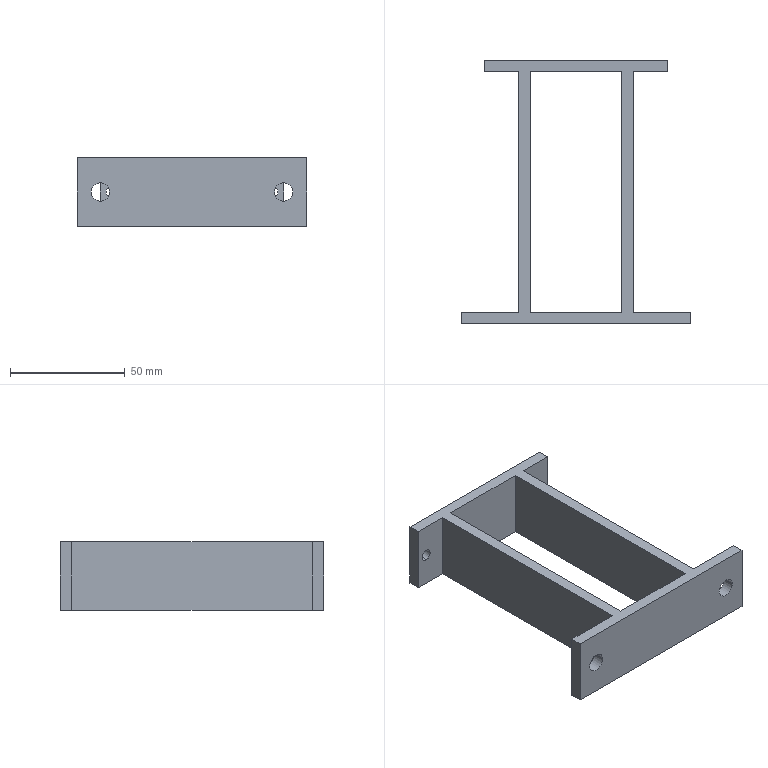Part | SolidWorks | features ICE 2, Extrusion 1 | 1 solid | 26 faces | box 100 x 115 x 30 mm | volume 57801 mm3 | plane 18 | cylinder 8 | commonest cylinder face diameters 5 x4 8 x4
STEP:
#1=CARTESIAN_POINT('',(85.,110.,12.5));
#2=VERTEX_POINT('',#1);
#3=CARTESIAN_POINT('',(85.,110.,17.5));
#4=VERTEX_POINT('',#3);
#5=CARTESIAN_POINT('',(85.,110.,15.));
#6=DIRECTION('',(0.,1.,0.));
#7=DIRECTION('',(0.,0.,1.));
#8=AXIS2_PLACEMENT_3D('',#5,#6,#7);
#9=CIRCLE('',#8,2.5);
#10=EDGE_CURVE('',#2,#4,#9,.T.);
#11=ORIENTED_EDGE('',*,*,#10,.F.);
#12=CARTESIAN_POINT('',(85.,115.,12.5));
#13=VERTEX_POINT('',#12);
#14=CARTESIAN_POINT('',(85.,105.,12.5));
#15=DIRECTION('',(0.,1.,0.));
#16=VECTOR('',#15,1000.);
#17=LINE('',#14,#16);
#18=EDGE_CURVE('',#2,#13,#17,.T.);
#19=ORIENTED_EDGE('',*,*,#18,.T.);
#20=CARTESIAN_POINT('',(85.,115.,17.5));
#21=VERTEX_POINT('',#20);
#22=CARTESIAN_POINT('',(85.,115.,15.));
#23=DIRECTION('',(0.,1.,0.));
#24=DIRECTION('',(0.,0.,1.));
#25=AXIS2_PLACEMENT_3D('',#22,#23,#24);
#26=CIRCLE('',#25,2.5);
#27=EDGE_CURVE('',#13,#21,#26,.T.);
#28=ORIENTED_EDGE('',*,*,#27,.T.);
#29=CARTESIAN_POINT('',(85.,105.,17.5));
#30=DIRECTION('',(0.,1.,0.));
#31=VECTOR('',#30,1000.);
#32=LINE('',#29,#31);
#33=EDGE_CURVE('',#4,#21,#32,.T.);
#34=ORIENTED_EDGE('',*,*,#33,.F.);
#35=EDGE_LOOP('',(#11,#19,#28,#34));
#36=FACE_OUTER_BOUND('',#35,.T.);
#37=CARTESIAN_POINT('',(85.,105.,15.));
#38=DIRECTION('',(0.,1.,0.));
#39=DIRECTION('',(0.,0.,1.));
#40=AXIS2_PLACEMENT_3D('',#37,#38,#39);
#41=CYLINDRICAL_SURFACE('',#40,2.5);
#42=ADVANCED_FACE('',(#36),#41,.F.);
#43=CARTESIAN_POINT('',(15.,110.,12.5));
#44=VERTEX_POINT('',#43);
#45=CARTESIAN_POINT('',(15.,110.,17.5));
#46=VERTEX_POINT('',#45);
#47=CARTESIAN_POINT('',(15.,110.,15.));
#48=DIRECTION('',(0.,1.,0.));
#49=DIRECTION('',(0.,0.,1.));
#50=AXIS2_PLACEMENT_3D('',#47,#48,#49);
#51=CIRCLE('',#50,2.5);
#52=EDGE_CURVE('',#44,#46,#51,.T.);
#53=ORIENTED_EDGE('',*,*,#52,.F.);
#54=CARTESIAN_POINT('',(15.,115.,12.5));
#55=VERTEX_POINT('',#54);
#56=CARTESIAN_POINT('',(15.,105.,12.5));
#57=DIRECTION('',(0.,1.,0.));
#58=VECTOR('',#57,1000.);
#59=LINE('',#56,#58);
#60=EDGE_CURVE('',#44,#55,#59,.T.);
#61=ORIENTED_EDGE('',*,*,#60,.T.);
#62=CARTESIAN_POINT('',(15.,115.,17.5));
#63=VERTEX_POINT('',#62);
#64=CARTESIAN_POINT('',(15.,115.,15.));
#65=DIRECTION('',(0.,1.,0.));
#66=DIRECTION('',(0.,0.,1.));
#67=AXIS2_PLACEMENT_3D('',#64,#65,#66);
#68=CIRCLE('',#67,2.5);
#69=EDGE_CURVE('',#55,#63,#68,.T.);
#70=ORIENTED_EDGE('',*,*,#69,.T.);
#71=CARTESIAN_POINT('',(15.,105.,17.5));
#72=DIRECTION('',(0.,1.,0.));
#73=VECTOR('',#72,1000.);
#74=LINE('',#71,#73);
#75=EDGE_CURVE('',#46,#63,#74,.T.);
#76=ORIENTED_EDGE('',*,*,#75,.F.);
#77=EDGE_LOOP('',(#53,#61,#70,#76));
#78=FACE_OUTER_BOUND('',#77,.T.);
#79=CARTESIAN_POINT('',(15.,105.,15.));
#80=DIRECTION('',(0.,1.,0.));
#81=DIRECTION('',(0.,0.,1.));
#82=AXIS2_PLACEMENT_3D('',#79,#80,#81);
#83=CYLINDRICAL_SURFACE('',#82,2.5);
#84=ADVANCED_FACE('',(#78),#83,.F.);
#85=CARTESIAN_POINT('',(14.,0.,15.));
#86=VERTEX_POINT('',#85);
#87=CARTESIAN_POINT('',(6.,0.,15.));
#88=VERTEX_POINT('',#87);
#89=CARTESIAN_POINT('',(10.,0.,15.));
#90=DIRECTION('',(0.,1.,0.));
#91=DIRECTION('',(-1.,0.,0.));
#92=AXIS2_PLACEMENT_3D('',#89,#90,#91);
#93=CIRCLE('',#92,4.);
#94=EDGE_CURVE('',#86,#88,#93,.T.);
#95=ORIENTED_EDGE('',*,*,#94,.F.);
#96=CARTESIAN_POINT('',(14.,5.,15.));
#97=VERTEX_POINT('',#96);
#98=CARTESIAN_POINT('',(14.,0.,15.));
#99=DIRECTION('',(0.,1.,0.));
#100=VECTOR('',#99,1000.);
#101=LINE('',#98,#100);
#102=EDGE_CURVE('',#86,#97,#101,.T.);
#103=ORIENTED_EDGE('',*,*,#102,.T.);
#104=CARTESIAN_POINT('',(6.,5.,15.));
#105=VERTEX_POINT('',#104);
#106=CARTESIAN_POINT('',(10.,5.,15.));
#107=DIRECTION('',(0.,1.,0.));
#108=DIRECTION('',(-1.,0.,0.));
#109=AXIS2_PLACEMENT_3D('',#106,#107,#108);
#110=CIRCLE('',#109,4.);
#111=EDGE_CURVE('',#97,#105,#110,.T.);
#112=ORIENTED_EDGE('',*,*,#111,.T.);
#113=CARTESIAN_POINT('',(6.,0.,15.));
#114=DIRECTION('',(0.,1.,0.));
#115=VECTOR('',#114,1000.);
#116=LINE('',#113,#115);
#117=EDGE_CURVE('',#88,#105,#116,.T.);
#118=ORIENTED_EDGE('',*,*,#117,.F.);
#119=EDGE_LOOP('',(#95,#103,#112,#118));
#120=FACE_OUTER_BOUND('',#119,.T.);
#121=CARTESIAN_POINT('',(10.,0.,15.));
#122=DIRECTION('',(0.,1.,0.));
#123=DIRECTION('',(-1.,0.,0.));
#124=AXIS2_PLACEMENT_3D('',#121,#122,#123);
#125=CYLINDRICAL_SURFACE('',#124,4.);
#126=ADVANCED_FACE('',(#120),#125,.F.);
#127=CARTESIAN_POINT('',(94.,0.,15.));
#128=VERTEX_POINT('',#127);
#129=CARTESIAN_POINT('',(86.,0.,15.));
#130=VERTEX_POINT('',#129);
#131=CARTESIAN_POINT('',(90.,0.,15.));
#132=DIRECTION('',(0.,1.,0.));
#133=DIRECTION('',(-1.,0.,0.));
#134=AXIS2_PLACEMENT_3D('',#131,#132,#133);
#135=CIRCLE('',#134,4.);
#136=EDGE_CURVE('',#128,#130,#135,.T.);
#137=ORIENTED_EDGE('',*,*,#136,.F.);
#138=CARTESIAN_POINT('',(94.,5.,15.));
#139=VERTEX_POINT('',#138);
#140=CARTESIAN_POINT('',(94.,0.,15.));
#141=DIRECTION('',(0.,1.,0.));
#142=VECTOR('',#141,1000.);
#143=LINE('',#140,#142);
#144=EDGE_CURVE('',#128,#139,#143,.T.);
#145=ORIENTED_EDGE('',*,*,#144,.T.);
#146=CARTESIAN_POINT('',(86.,5.,15.));
#147=VERTEX_POINT('',#146);
#148=CARTESIAN_POINT('',(90.,5.,15.));
#149=DIRECTION('',(0.,1.,0.));
#150=DIRECTION('',(-1.,0.,0.));
#151=AXIS2_PLACEMENT_3D('',#148,#149,#150);
#152=CIRCLE('',#151,4.);
#153=EDGE_CURVE('',#139,#147,#152,.T.);
#154=ORIENTED_EDGE('',*,*,#153,.T.);
#155=CARTESIAN_POINT('',(86.,0.,15.));
#156=DIRECTION('',(0.,1.,0.));
#157=VECTOR('',#156,1000.);
#158=LINE('',#155,#157);
#159=EDGE_CURVE('',#130,#147,#158,.T.);
#160=ORIENTED_EDGE('',*,*,#159,.F.);
#161=EDGE_LOOP('',(#137,#145,#154,#160));
#162=FACE_OUTER_BOUND('',#161,.T.);
#163=CARTESIAN_POINT('',(90.,0.,15.));
#164=DIRECTION('',(0.,1.,0.));
#165=DIRECTION('',(-1.,0.,0.));
#166=AXIS2_PLACEMENT_3D('',#163,#164,#165);
#167=CYLINDRICAL_SURFACE('',#166,4.);
#168=ADVANCED_FACE('',(#162),#167,.F.);
#169=CARTESIAN_POINT('',(0.,5.,30.));
#170=VERTEX_POINT('',#169);
#171=CARTESIAN_POINT('',(0.,0.,30.));
#172=VERTEX_POINT('',#171);
#173=CARTESIAN_POINT('',(0.,5.,30.));
#174=DIRECTION('',(0.,-1.,0.));
#175=VECTOR('',#174,1000.);
#176=LINE('',#173,#175);
#177=EDGE_CURVE('',#170,#172,#176,.T.);
#178=ORIENTED_EDGE('',*,*,#177,.T.);
#179=CARTESIAN_POINT('',(100.,0.,30.));
#180=VERTEX_POINT('',#179);
#181=CARTESIAN_POINT('',(0.,0.,30.));
#182=DIRECTION('',(1.,0.,0.));
#183=VECTOR('',#182,1000.);
#184=LINE('',#181,#183);
#185=EDGE_CURVE('',#172,#180,#184,.T.);
#186=ORIENTED_EDGE('',*,*,#185,.T.);
#187=CARTESIAN_POINT('',(100.,5.,30.));
#188=VERTEX_POINT('',#187);
#189=CARTESIAN_POINT('',(100.,0.,30.));
#190=DIRECTION('',(0.,1.,0.));
#191=VECTOR('',#190,1000.);
#192=LINE('',#189,#191);
#193=EDGE_CURVE('',#180,#188,#192,.T.);
#194=ORIENTED_EDGE('',*,*,#193,.T.);
#195=CARTESIAN_POINT('',(75.,5.,30.));
#196=VERTEX_POINT('',#195);
#197=CARTESIAN_POINT('',(100.,5.,30.));
#198=DIRECTION('',(-1.,0.,0.));
#199=VECTOR('',#198,1000.);
#200=LINE('',#197,#199);
#201=EDGE_CURVE('',#188,#196,#200,.T.);
#202=ORIENTED_EDGE('',*,*,#201,.T.);
#203=CARTESIAN_POINT('',(75.,110.,30.));
#204=VERTEX_POINT('',#203);
#205=CARTESIAN_POINT('',(75.,5.,30.));
#206=DIRECTION('',(0.,1.,0.));
#207=VECTOR('',#206,1000.);
#208=LINE('',#205,#207);
#209=EDGE_CURVE('',#196,#204,#208,.T.);
#210=ORIENTED_EDGE('',*,*,#209,.T.);
#211=CARTESIAN_POINT('',(90.,110.,30.));
#212=VERTEX_POINT('',#211);
#213=CARTESIAN_POINT('',(75.,110.,30.));
#214=DIRECTION('',(1.,0.,0.));
#215=VECTOR('',#214,1000.);
#216=LINE('',#213,#215);
#217=EDGE_CURVE('',#204,#212,#216,.T.);
#218=ORIENTED_EDGE('',*,*,#217,.T.);
#219=CARTESIAN_POINT('',(90.,115.,30.));
#220=VERTEX_POINT('',#219);
#221=CARTESIAN_POINT('',(90.,110.,30.));
#222=DIRECTION('',(0.,1.,0.));
#223=VECTOR('',#222,1000.);
#224=LINE('',#221,#223);
#225=EDGE_CURVE('',#212,#220,#224,.T.);
#226=ORIENTED_EDGE('',*,*,#225,.T.);
#227=CARTESIAN_POINT('',(10.,115.,30.));
#228=VERTEX_POINT('',#227);
#229=CARTESIAN_POINT('',(90.,115.,30.));
#230=DIRECTION('',(-1.,0.,0.));
#231=VECTOR('',#230,1000.);
#232=LINE('',#229,#231);
#233=EDGE_CURVE('',#220,#228,#232,.T.);
#234=ORIENTED_EDGE('',*,*,#233,.T.);
#235=CARTESIAN_POINT('',(10.,110.,30.));
#236=VERTEX_POINT('',#235);
#237=CARTESIAN_POINT('',(10.,115.,30.));
#238=DIRECTION('',(0.,-1.,0.));
#239=VECTOR('',#238,1000.);
#240=LINE('',#237,#239);
#241=EDGE_CURVE('',#228,#236,#240,.T.);
#242=ORIENTED_EDGE('',*,*,#241,.T.);
#243=CARTESIAN_POINT('',(25.,110.,30.));
#244=VERTEX_POINT('',#243);
#245=CARTESIAN_POINT('',(10.,110.,30.));
#246=DIRECTION('',(1.,0.,0.));
#247=VECTOR('',#246,1000.);
#248=LINE('',#245,#247);
#249=EDGE_CURVE('',#236,#244,#248,.T.);
#250=ORIENTED_EDGE('',*,*,#249,.T.);
#251=CARTESIAN_POINT('',(25.,5.,30.));
#252=VERTEX_POINT('',#251);
#253=CARTESIAN_POINT('',(25.,110.,30.));
#254=DIRECTION('',(0.,-1.,0.));
#255=VECTOR('',#254,1000.);
#256=LINE('',#253,#255);
#257=EDGE_CURVE('',#244,#252,#256,.T.);
#258=ORIENTED_EDGE('',*,*,#257,.T.);
#259=CARTESIAN_POINT('',(25.,5.,30.));
#260=DIRECTION('',(-1.,0.,0.));
#261=VECTOR('',#260,1000.);
#262=LINE('',#259,#261);
#263=EDGE_CURVE('',#252,#170,#262,.T.);
#264=ORIENTED_EDGE('',*,*,#263,.T.);
#265=EDGE_LOOP('',(#178,#186,#194,#202,#210,#218,#226,#234,#242,#250,#258,#264));
#266=FACE_OUTER_BOUND('',#265,.T.);
#267=CARTESIAN_POINT('',(30.,5.,30.));
#268=VERTEX_POINT('',#267);
#269=CARTESIAN_POINT('',(70.,5.,30.));
#270=VERTEX_POINT('',#269);
#271=CARTESIAN_POINT('',(30.,5.,30.));
#272=DIRECTION('',(1.,0.,0.));
#273=VECTOR('',#272,1000.);
#274=LINE('',#271,#273);
#275=EDGE_CURVE('',#268,#270,#274,.T.);
#276=ORIENTED_EDGE('',*,*,#275,.F.);
#277=CARTESIAN_POINT('',(30.,110.,30.));
#278=VERTEX_POINT('',#277);
#279=CARTESIAN_POINT('',(30.,110.,30.));
#280=DIRECTION('',(0.,-1.,0.));
#281=VECTOR('',#280,1000.);
#282=LINE('',#279,#281);
#283=EDGE_CURVE('',#278,#268,#282,.T.);
#284=ORIENTED_EDGE('',*,*,#283,.F.);
#285=CARTESIAN_POINT('',(70.,110.,30.));
#286=VERTEX_POINT('',#285);
#287=CARTESIAN_POINT('',(30.,110.,30.));
#288=DIRECTION('',(-1.,0.,0.));
#289=VECTOR('',#288,1000.);
#290=LINE('',#287,#289);
#291=EDGE_CURVE('',#286,#278,#290,.T.);
#292=ORIENTED_EDGE('',*,*,#291,.F.);
#293=CARTESIAN_POINT('',(70.,110.,30.));
#294=DIRECTION('',(0.,1.,0.));
#295=VECTOR('',#294,1000.);
#296=LINE('',#293,#295);
#297=EDGE_CURVE('',#270,#286,#296,.T.);
#298=ORIENTED_EDGE('',*,*,#297,.F.);
#299=EDGE_LOOP('',(#276,#284,#292,#298));
#300=FACE_BOUND('',#299,.T.);
#301=CARTESIAN_POINT('',(0.,0.,30.));
#302=DIRECTION('',(0.,0.,1.));
#303=DIRECTION('',(1.,0.,0.));
#304=AXIS2_PLACEMENT_3D('',#301,#302,#303);
#305=PLANE('',#304);
#306=ADVANCED_FACE('',(#266,#300),#305,.T.);
#307=CARTESIAN_POINT('',(0.,5.,0.));
#308=VERTEX_POINT('',#307);
#309=CARTESIAN_POINT('',(0.,0.,0.));
#310=VERTEX_POINT('',#309);
#311=CARTESIAN_POINT('',(0.,5.,0.));
#312=DIRECTION('',(0.,-1.,0.));
#313=VECTOR('',#312,1000.);
#314=LINE('',#311,#313);
#315=EDGE_CURVE('',#308,#310,#314,.T.);
#316=ORIENTED_EDGE('',*,*,#315,.F.);
#317=CARTESIAN_POINT('',(25.,5.,0.));
#318=VERTEX_POINT('',#317);
#319=CARTESIAN_POINT('',(25.,5.,0.));
#320=DIRECTION('',(-1.,0.,0.));
#321=VECTOR('',#320,1000.);
#322=LINE('',#319,#321);
#323=EDGE_CURVE('',#318,#308,#322,.T.);
#324=ORIENTED_EDGE('',*,*,#323,.F.);
#325=CARTESIAN_POINT('',(25.,110.,0.));
#326=VERTEX_POINT('',#325);
#327=CARTESIAN_POINT('',(25.,110.,0.));
#328=DIRECTION('',(0.,-1.,0.));
#329=VECTOR('',#328,1000.);
#330=LINE('',#327,#329);
#331=EDGE_CURVE('',#326,#318,#330,.T.);
#332=ORIENTED_EDGE('',*,*,#331,.F.);
#333=CARTESIAN_POINT('',(10.,110.,0.));
#334=VERTEX_POINT('',#333);
#335=CARTESIAN_POINT('',(10.,110.,0.));
#336=DIRECTION('',(1.,0.,0.));
#337=VECTOR('',#336,1000.);
#338=LINE('',#335,#337);
#339=EDGE_CURVE('',#334,#326,#338,.T.);
#340=ORIENTED_EDGE('',*,*,#339,.F.);
#341=CARTESIAN_POINT('',(10.,115.,0.));
#342=VERTEX_POINT('',#341);
#343=CARTESIAN_POINT('',(10.,115.,0.));
#344=DIRECTION('',(0.,-1.,0.));
#345=VECTOR('',#344,1000.);
#346=LINE('',#343,#345);
#347=EDGE_CURVE('',#342,#334,#346,.T.);
#348=ORIENTED_EDGE('',*,*,#347,.F.);
#349=CARTESIAN_POINT('',(90.,115.,0.));
#350=VERTEX_POINT('',#349);
#351=CARTESIAN_POINT('',(90.,115.,0.));
#352=DIRECTION('',(-1.,0.,0.));
#353=VECTOR('',#352,1000.);
#354=LINE('',#351,#353);
#355=EDGE_CURVE('',#350,#342,#354,.T.);
#356=ORIENTED_EDGE('',*,*,#355,.F.);
#357=CARTESIAN_POINT('',(90.,110.,0.));
#358=VERTEX_POINT('',#357);
#359=CARTESIAN_POINT('',(90.,110.,0.));
#360=DIRECTION('',(0.,1.,0.));
#361=VECTOR('',#360,1000.);
#362=LINE('',#359,#361);
#363=EDGE_CURVE('',#358,#350,#362,.T.);
#364=ORIENTED_EDGE('',*,*,#363,.F.);
#365=CARTESIAN_POINT('',(75.,110.,0.));
#366=VERTEX_POINT('',#365);
#367=CARTESIAN_POINT('',(75.,110.,0.));
#368=DIRECTION('',(1.,0.,0.));
#369=VECTOR('',#368,1000.);
#370=LINE('',#367,#369);
#371=EDGE_CURVE('',#366,#358,#370,.T.);
#372=ORIENTED_EDGE('',*,*,#371,.F.);
#373=CARTESIAN_POINT('',(75.,5.,0.));
#374=VERTEX_POINT('',#373);
#375=CARTESIAN_POINT('',(75.,5.,0.));
#376=DIRECTION('',(0.,1.,0.));
#377=VECTOR('',#376,1000.);
#378=LINE('',#375,#377);
#379=EDGE_CURVE('',#374,#366,#378,.T.);
#380=ORIENTED_EDGE('',*,*,#379,.F.);
#381=CARTESIAN_POINT('',(100.,5.,0.));
#382=VERTEX_POINT('',#381);
#383=CARTESIAN_POINT('',(100.,5.,0.));
#384=DIRECTION('',(-1.,0.,0.));
#385=VECTOR('',#384,1000.);
#386=LINE('',#383,#385);
#387=EDGE_CURVE('',#382,#374,#386,.T.);
#388=ORIENTED_EDGE('',*,*,#387,.F.);
#389=CARTESIAN_POINT('',(100.,0.,0.));
#390=VERTEX_POINT('',#389);
#391=CARTESIAN_POINT('',(100.,0.,0.));
#392=DIRECTION('',(0.,1.,0.));
#393=VECTOR('',#392,1000.);
#394=LINE('',#391,#393);
#395=EDGE_CURVE('',#390,#382,#394,.T.);
#396=ORIENTED_EDGE('',*,*,#395,.F.);
#397=CARTESIAN_POINT('',(0.,0.,0.));
#398=DIRECTION('',(1.,0.,0.));
#399=VECTOR('',#398,1000.);
#400=LINE('',#397,#399);
#401=EDGE_CURVE('',#310,#390,#400,.T.);
#402=ORIENTED_EDGE('',*,*,#401,.F.);
#403=EDGE_LOOP('',(#316,#324,#332,#340,#348,#356,#364,#372,#380,#388,#396,#402));
#404=FACE_OUTER_BOUND('',#403,.T.);
#405=CARTESIAN_POINT('',(30.,110.,0.));
#406=VERTEX_POINT('',#405);
#407=CARTESIAN_POINT('',(30.,5.,0.));
#408=VERTEX_POINT('',#407);
#409=CARTESIAN_POINT('',(30.,110.,0.));
#410=DIRECTION('',(0.,-1.,0.));
#411=VECTOR('',#410,1000.);
#412=LINE('',#409,#411);
#413=EDGE_CURVE('',#406,#408,#412,.T.);
#414=ORIENTED_EDGE('',*,*,#413,.T.);
#415=CARTESIAN_POINT('',(70.,5.,0.));
#416=VERTEX_POINT('',#415);
#417=CARTESIAN_POINT('',(30.,5.,0.));
#418=DIRECTION('',(1.,0.,0.));
#419=VECTOR('',#418,1000.);
#420=LINE('',#417,#419);
#421=EDGE_CURVE('',#408,#416,#420,.T.);
#422=ORIENTED_EDGE('',*,*,#421,.T.);
#423=CARTESIAN_POINT('',(70.,110.,0.));
#424=VERTEX_POINT('',#423);
#425=CARTESIAN_POINT('',(70.,110.,0.));
#426=DIRECTION('',(0.,1.,0.));
#427=VECTOR('',#426,1000.);
#428=LINE('',#425,#427);
#429=EDGE_CURVE('',#416,#424,#428,.T.);
#430=ORIENTED_EDGE('',*,*,#429,.T.);
#431=CARTESIAN_POINT('',(30.,110.,0.));
#432=DIRECTION('',(-1.,0.,0.));
#433=VECTOR('',#432,1000.);
#434=LINE('',#431,#433);
#435=EDGE_CURVE('',#424,#406,#434,.T.);
#436=ORIENTED_EDGE('',*,*,#435,.T.);
#437=EDGE_LOOP('',(#414,#422,#430,#436));
#438=FACE_BOUND('',#437,.T.);
#439=CARTESIAN_POINT('',(0.,0.,0.));
#440=DIRECTION('',(0.,0.,1.));
#441=DIRECTION('',(1.,0.,0.));
#442=AXIS2_PLACEMENT_3D('',#439,#440,#441);
#443=PLANE('',#442);
#444=ADVANCED_FACE('',(#404,#438),#443,.F.);
#445=ORIENTED_EDGE('',*,*,#315,.T.);
#446=CARTESIAN_POINT('',(0.,0.,30.));
#447=DIRECTION('',(0.,0.,-1.));
#448=VECTOR('',#447,1000.);
#449=LINE('',#446,#448);
#450=EDGE_CURVE('',#172,#310,#449,.T.);
#451=ORIENTED_EDGE('',*,*,#450,.F.);
#452=ORIENTED_EDGE('',*,*,#177,.F.);
#453=CARTESIAN_POINT('',(0.,5.,30.));
#454=DIRECTION('',(0.,0.,-1.));
#455=VECTOR('',#454,1000.);
#456=LINE('',#453,#455);
#457=EDGE_CURVE('',#170,#308,#456,.T.);
#458=ORIENTED_EDGE('',*,*,#457,.T.);
#459=EDGE_LOOP('',(#445,#451,#452,#458));
#460=FACE_OUTER_BOUND('',#459,.T.);
#461=CARTESIAN_POINT('',(0.,5.,30.));
#462=DIRECTION('',(1.,0.,0.));
#463=DIRECTION('',(0.,1.,0.));
#464=AXIS2_PLACEMENT_3D('',#461,#462,#463);
#465=PLANE('',#464);
#466=ADVANCED_FACE('',(#460),#465,.F.);
#467=CARTESIAN_POINT('',(10.,0.,15.));
#468=DIRECTION('',(0.,1.,0.));
#469=DIRECTION('',(-1.,0.,0.));
#470=AXIS2_PLACEMENT_3D('',#467,#468,#469);
#471=CIRCLE('',#470,4.);
#472=EDGE_CURVE('',#88,#86,#471,.T.);
#473=ORIENTED_EDGE('',*,*,#472,.T.);
#474=ORIENTED_EDGE('',*,*,#94,.T.);
#475=EDGE_LOOP('',(#473,#474));
#476=FACE_BOUND('',#475,.T.);
#477=CARTESIAN_POINT('',(90.,0.,15.));
#478=DIRECTION('',(0.,1.,0.));
#479=DIRECTION('',(-1.,0.,0.));
#480=AXIS2_PLACEMENT_3D('',#477,#478,#479);
#481=CIRCLE('',#480,4.);
#482=EDGE_CURVE('',#130,#128,#481,.T.);
#483=ORIENTED_EDGE('',*,*,#482,.T.);
#484=ORIENTED_EDGE('',*,*,#136,.T.);
#485=EDGE_LOOP('',(#483,#484));
#486=FACE_BOUND('',#485,.T.);
#487=ORIENTED_EDGE('',*,*,#401,.T.);
#488=CARTESIAN_POINT('',(100.,0.,30.));
#489=DIRECTION('',(0.,0.,-1.));
#490=VECTOR('',#489,1000.);
#491=LINE('',#488,#490);
#492=EDGE_CURVE('',#180,#390,#491,.T.);
#493=ORIENTED_EDGE('',*,*,#492,.F.);
#494=ORIENTED_EDGE('',*,*,#185,.F.);
#495=ORIENTED_EDGE('',*,*,#450,.T.);
#496=EDGE_LOOP('',(#487,#493,#494,#495));
#497=FACE_OUTER_BOUND('',#496,.T.);
#498=CARTESIAN_POINT('',(0.,0.,30.));
#499=DIRECTION('',(0.,1.,0.));
#500=DIRECTION('',(0.,0.,1.));
#501=AXIS2_PLACEMENT_3D('',#498,#499,#500);
#502=PLANE('',#501);
#503=ADVANCED_FACE('',(#476,#486,#497),#502,.F.);
#504=ORIENTED_EDGE('',*,*,#395,.T.);
#505=CARTESIAN_POINT('',(100.,5.,30.));
#506=DIRECTION('',(0.,0.,-1.));
#507=VECTOR('',#506,1000.);
#508=LINE('',#505,#507);
#509=EDGE_CURVE('',#188,#382,#508,.T.);
#510=ORIENTED_EDGE('',*,*,#509,.F.);
#511=ORIENTED_EDGE('',*,*,#193,.F.);
#512=ORIENTED_EDGE('',*,*,#492,.T.);
#513=EDGE_LOOP('',(#504,#510,#511,#512));
#514=FACE_OUTER_BOUND('',#513,.T.);
#515=CARTESIAN_POINT('',(100.,0.,30.));
#516=DIRECTION('',(-1.,0.,0.));
#517=DIRECTION('',(0.,0.,1.));
#518=AXIS2_PLACEMENT_3D('',#515,#516,#517);
#519=PLANE('',#518);
#520=ADVANCED_FACE('',(#514),#519,.F.);
#521=CARTESIAN_POINT('',(90.,5.,15.));
#522=DIRECTION('',(0.,1.,0.));
#523=DIRECTION('',(-1.,0.,0.));
#524=AXIS2_PLACEMENT_3D('',#521,#522,#523);
#525=CIRCLE('',#524,4.);
#526=EDGE_CURVE('',#147,#139,#525,.T.);
#527=ORIENTED_EDGE('',*,*,#526,.F.);
#528=ORIENTED_EDGE('',*,*,#153,.F.);
#529=EDGE_LOOP('',(#527,#528));
#530=FACE_BOUND('',#529,.T.);
#531=ORIENTED_EDGE('',*,*,#387,.T.);
#532=CARTESIAN_POINT('',(75.,5.,30.));
#533=DIRECTION('',(0.,0.,-1.));
#534=VECTOR('',#533,1000.);
#535=LINE('',#532,#534);
#536=EDGE_CURVE('',#196,#374,#535,.T.);
#537=ORIENTED_EDGE('',*,*,#536,.F.);
#538=ORIENTED_EDGE('',*,*,#201,.F.);
#539=ORIENTED_EDGE('',*,*,#509,.T.);
#540=EDGE_LOOP('',(#531,#537,#538,#539));
#541=FACE_OUTER_BOUND('',#540,.T.);
#542=CARTESIAN_POINT('',(100.,5.,30.));
#543=DIRECTION('',(0.,-1.,0.));
#544=DIRECTION('',(1.,0.,0.));
#545=AXIS2_PLACEMENT_3D('',#542,#543,#544);
#546=PLANE('',#545);
#547=ADVANCED_FACE('',(#530,#541),#546,.F.);
#548=ORIENTED_EDGE('',*,*,#379,.T.);
#549=CARTESIAN_POINT('',(75.,110.,30.));
#550=DIRECTION('',(0.,0.,-1.));
#551=VECTOR('',#550,1000.);
#552=LINE('',#549,#551);
#553=EDGE_CURVE('',#204,#366,#552,.T.);
#554=ORIENTED_EDGE('',*,*,#553,.F.);
#555=ORIENTED_EDGE('',*,*,#209,.F.);
#556=ORIENTED_EDGE('',*,*,#536,.T.);
#557=EDGE_LOOP('',(#548,#554,#555,#556));
#558=FACE_OUTER_BOUND('',#557,.T.);
#559=CARTESIAN_POINT('',(75.,5.,30.));
#560=DIRECTION('',(-1.,0.,0.));
#561=DIRECTION('',(0.,0.,1.));
#562=AXIS2_PLACEMENT_3D('',#559,#560,#561);
#563=PLANE('',#562);
#564=ADVANCED_FACE('',(#558),#563,.F.);
#565=CARTESIAN_POINT('',(85.,110.,15.));
#566=DIRECTION('',(0.,1.,0.));
#567=DIRECTION('',(0.,0.,1.));
#568=AXIS2_PLACEMENT_3D('',#565,#566,#567);
#569=CIRCLE('',#568,2.5);
#570=EDGE_CURVE('',#4,#2,#569,.T.);
#571=ORIENTED_EDGE('',*,*,#570,.T.);
#572=ORIENTED_EDGE('',*,*,#10,.T.);
#573=EDGE_LOOP('',(#571,#572));
#574=FACE_BOUND('',#573,.T.);
#575=ORIENTED_EDGE('',*,*,#371,.T.);
#576=CARTESIAN_POINT('',(90.,110.,30.));
#577=DIRECTION('',(0.,0.,-1.));
#578=VECTOR('',#577,1000.);
#579=LINE('',#576,#578);
#580=EDGE_CURVE('',#212,#358,#579,.T.);
#581=ORIENTED_EDGE('',*,*,#580,.F.);
#582=ORIENTED_EDGE('',*,*,#217,.F.);
#583=ORIENTED_EDGE('',*,*,#553,.T.);
#584=EDGE_LOOP('',(#575,#581,#582,#583));
#585=FACE_OUTER_BOUND('',#584,.T.);
#586=CARTESIAN_POINT('',(75.,110.,30.));
#587=DIRECTION('',(0.,1.,0.));
#588=DIRECTION('',(0.,0.,1.));
#589=AXIS2_PLACEMENT_3D('',#586,#587,#588);
#590=PLANE('',#589);
#591=ADVANCED_FACE('',(#574,#585),#590,.F.);
#592=ORIENTED_EDGE('',*,*,#363,.T.);
#593=CARTESIAN_POINT('',(90.,115.,30.));
#594=DIRECTION('',(0.,0.,-1.));
#595=VECTOR('',#594,1000.);
#596=LINE('',#593,#595);
#597=EDGE_CURVE('',#220,#350,#596,.T.);
#598=ORIENTED_EDGE('',*,*,#597,.F.);
#599=ORIENTED_EDGE('',*,*,#225,.F.);
#600=ORIENTED_EDGE('',*,*,#580,.T.);
#601=EDGE_LOOP('',(#592,#598,#599,#600));
#602=FACE_OUTER_BOUND('',#601,.T.);
#603=CARTESIAN_POINT('',(90.,110.,30.));
#604=DIRECTION('',(-1.,0.,0.));
#605=DIRECTION('',(0.,0.,1.));
#606=AXIS2_PLACEMENT_3D('',#603,#604,#605);
#607=PLANE('',#606);
#608=ADVANCED_FACE('',(#602),#607,.F.);
#609=CARTESIAN_POINT('',(85.,115.,15.));
#610=DIRECTION('',(0.,1.,0.));
#611=DIRECTION('',(0.,0.,1.));
#612=AXIS2_PLACEMENT_3D('',#609,#610,#611);
#613=CIRCLE('',#612,2.5);
#614=EDGE_CURVE('',#21,#13,#613,.T.);
#615=ORIENTED_EDGE('',*,*,#614,.F.);
#616=ORIENTED_EDGE('',*,*,#27,.F.);
#617=EDGE_LOOP('',(#615,#616));
#618=FACE_BOUND('',#617,.T.);
#619=CARTESIAN_POINT('',(15.,115.,15.));
#620=DIRECTION('',(0.,1.,0.));
#621=DIRECTION('',(0.,0.,1.));
#622=AXIS2_PLACEMENT_3D('',#619,#620,#621);
#623=CIRCLE('',#622,2.5);
#624=EDGE_CURVE('',#63,#55,#623,.T.);
#625=ORIENTED_EDGE('',*,*,#624,.F.);
#626=ORIENTED_EDGE('',*,*,#69,.F.);
#627=EDGE_LOOP('',(#625,#626));
#628=FACE_BOUND('',#627,.T.);
#629=ORIENTED_EDGE('',*,*,#355,.T.);
#630=CARTESIAN_POINT('',(10.,115.,30.));
#631=DIRECTION('',(0.,0.,-1.));
#632=VECTOR('',#631,1000.);
#633=LINE('',#630,#632);
#634=EDGE_CURVE('',#228,#342,#633,.T.);
#635=ORIENTED_EDGE('',*,*,#634,.F.);
#636=ORIENTED_EDGE('',*,*,#233,.F.);
#637=ORIENTED_EDGE('',*,*,#597,.T.);
#638=EDGE_LOOP('',(#629,#635,#636,#637));
#639=FACE_OUTER_BOUND('',#638,.T.);
#640=CARTESIAN_POINT('',(90.,115.,30.));
#641=DIRECTION('',(0.,-1.,0.));
#642=DIRECTION('',(0.,0.,-1.));
#643=AXIS2_PLACEMENT_3D('',#640,#641,#642);
#644=PLANE('',#643);
#645=ADVANCED_FACE('',(#618,#628,#639),#644,.F.);
#646=ORIENTED_EDGE('',*,*,#347,.T.);
#647=CARTESIAN_POINT('',(10.,110.,30.));
#648=DIRECTION('',(0.,0.,-1.));
#649=VECTOR('',#648,1000.);
#650=LINE('',#647,#649);
#651=EDGE_CURVE('',#236,#334,#650,.T.);
#652=ORIENTED_EDGE('',*,*,#651,.F.);
#653=ORIENTED_EDGE('',*,*,#241,.F.);
#654=ORIENTED_EDGE('',*,*,#634,.T.);
#655=EDGE_LOOP('',(#646,#652,#653,#654));
#656=FACE_OUTER_BOUND('',#655,.T.);
#657=CARTESIAN_POINT('',(10.,115.,30.));
#658=DIRECTION('',(1.,0.,0.));
#659=DIRECTION('',(0.,0.,-1.));
#660=AXIS2_PLACEMENT_3D('',#657,#658,#659);
#661=PLANE('',#660);
#662=ADVANCED_FACE('',(#656),#661,.F.);
#663=CARTESIAN_POINT('',(15.,110.,15.));
#664=DIRECTION('',(0.,1.,0.));
#665=DIRECTION('',(0.,0.,1.));
#666=AXIS2_PLACEMENT_3D('',#663,#664,#665);
#667=CIRCLE('',#666,2.5);
#668=EDGE_CURVE('',#46,#44,#667,.T.);
#669=ORIENTED_EDGE('',*,*,#668,.T.);
#670=ORIENTED_EDGE('',*,*,#52,.T.);
#671=EDGE_LOOP('',(#669,#670));
#672=FACE_BOUND('',#671,.T.);
#673=ORIENTED_EDGE('',*,*,#339,.T.);
#674=CARTESIAN_POINT('',(25.,110.,30.));
#675=DIRECTION('',(0.,0.,-1.));
#676=VECTOR('',#675,1000.);
#677=LINE('',#674,#676);
#678=EDGE_CURVE('',#244,#326,#677,.T.);
#679=ORIENTED_EDGE('',*,*,#678,.F.);
#680=ORIENTED_EDGE('',*,*,#249,.F.);
#681=ORIENTED_EDGE('',*,*,#651,.T.);
#682=EDGE_LOOP('',(#673,#679,#680,#681));
#683=FACE_OUTER_BOUND('',#682,.T.);
#684=CARTESIAN_POINT('',(10.,110.,30.));
#685=DIRECTION('',(0.,1.,0.));
#686=DIRECTION('',(0.,0.,1.));
#687=AXIS2_PLACEMENT_3D('',#684,#685,#686);
#688=PLANE('',#687);
#689=ADVANCED_FACE('',(#672,#683),#688,.F.);
#690=ORIENTED_EDGE('',*,*,#331,.T.);
#691=CARTESIAN_POINT('',(25.,5.,30.));
#692=DIRECTION('',(0.,0.,-1.));
#693=VECTOR('',#692,1000.);
#694=LINE('',#691,#693);
#695=EDGE_CURVE('',#252,#318,#694,.T.);
#696=ORIENTED_EDGE('',*,*,#695,.F.);
#697=ORIENTED_EDGE('',*,*,#257,.F.);
#698=ORIENTED_EDGE('',*,*,#678,.T.);
#699=EDGE_LOOP('',(#690,#696,#697,#698));
#700=FACE_OUTER_BOUND('',#699,.T.);
#701=CARTESIAN_POINT('',(25.,110.,30.));
#702=DIRECTION('',(1.,0.,0.));
#703=DIRECTION('',(0.,1.,0.));
#704=AXIS2_PLACEMENT_3D('',#701,#702,#703);
#705=PLANE('',#704);
#706=ADVANCED_FACE('',(#700),#705,.F.);
#707=CARTESIAN_POINT('',(10.,5.,15.));
#708=DIRECTION('',(0.,1.,0.));
#709=DIRECTION('',(-1.,0.,0.));
#710=AXIS2_PLACEMENT_3D('',#707,#708,#709);
#711=CIRCLE('',#710,4.);
#712=EDGE_CURVE('',#105,#97,#711,.T.);
#713=ORIENTED_EDGE('',*,*,#712,.F.);
#714=ORIENTED_EDGE('',*,*,#111,.F.);
#715=EDGE_LOOP('',(#713,#714));
#716=FACE_BOUND('',#715,.T.);
#717=ORIENTED_EDGE('',*,*,#323,.T.);
#718=ORIENTED_EDGE('',*,*,#457,.F.);
#719=ORIENTED_EDGE('',*,*,#263,.F.);
#720=ORIENTED_EDGE('',*,*,#695,.T.);
#721=EDGE_LOOP('',(#717,#718,#719,#720));
#722=FACE_OUTER_BOUND('',#721,.T.);
#723=CARTESIAN_POINT('',(25.,5.,30.));
#724=DIRECTION('',(0.,-1.,0.));
#725=DIRECTION('',(1.,0.,0.));
#726=AXIS2_PLACEMENT_3D('',#723,#724,#725);
#727=PLANE('',#726);
#728=ADVANCED_FACE('',(#716,#722),#727,.F.);
#729=ORIENTED_EDGE('',*,*,#413,.F.);
#730=CARTESIAN_POINT('',(30.,110.,30.));
#731=DIRECTION('',(0.,0.,-1.));
#732=VECTOR('',#731,1000.);
#733=LINE('',#730,#732);
#734=EDGE_CURVE('',#278,#406,#733,.T.);
#735=ORIENTED_EDGE('',*,*,#734,.F.);
#736=ORIENTED_EDGE('',*,*,#283,.T.);
#737=CARTESIAN_POINT('',(30.,5.,30.));
#738=DIRECTION('',(0.,0.,-1.));
#739=VECTOR('',#738,1000.);
#740=LINE('',#737,#739);
#741=EDGE_CURVE('',#268,#408,#740,.T.);
#742=ORIENTED_EDGE('',*,*,#741,.T.);
#743=EDGE_LOOP('',(#729,#735,#736,#742));
#744=FACE_OUTER_BOUND('',#743,.T.);
#745=CARTESIAN_POINT('',(30.,110.,30.));
#746=DIRECTION('',(1.,0.,0.));
#747=DIRECTION('',(0.,1.,0.));
#748=AXIS2_PLACEMENT_3D('',#745,#746,#747);
#749=PLANE('',#748);
#750=ADVANCED_FACE('',(#744),#749,.T.);
#751=ORIENTED_EDGE('',*,*,#421,.F.);
#752=ORIENTED_EDGE('',*,*,#741,.F.);
#753=ORIENTED_EDGE('',*,*,#275,.T.);
#754=CARTESIAN_POINT('',(70.,5.,30.));
#755=DIRECTION('',(0.,0.,-1.));
#756=VECTOR('',#755,1000.);
#757=LINE('',#754,#756);
#758=EDGE_CURVE('',#270,#416,#757,.T.);
#759=ORIENTED_EDGE('',*,*,#758,.T.);
#760=EDGE_LOOP('',(#751,#752,#753,#759));
#761=FACE_OUTER_BOUND('',#760,.T.);
#762=CARTESIAN_POINT('',(30.,5.,30.));
#763=DIRECTION('',(0.,1.,0.));
#764=DIRECTION('',(0.,0.,1.));
#765=AXIS2_PLACEMENT_3D('',#762,#763,#764);
#766=PLANE('',#765);
#767=ADVANCED_FACE('',(#761),#766,.T.);
#768=ORIENTED_EDGE('',*,*,#429,.F.);
#769=ORIENTED_EDGE('',*,*,#758,.F.);
#770=ORIENTED_EDGE('',*,*,#297,.T.);
#771=CARTESIAN_POINT('',(70.,110.,30.));
#772=DIRECTION('',(0.,0.,-1.));
#773=VECTOR('',#772,1000.);
#774=LINE('',#771,#773);
#775=EDGE_CURVE('',#286,#424,#774,.T.);
#776=ORIENTED_EDGE('',*,*,#775,.T.);
#777=EDGE_LOOP('',(#768,#769,#770,#776));
#778=FACE_OUTER_BOUND('',#777,.T.);
#779=CARTESIAN_POINT('',(70.,110.,30.));
#780=DIRECTION('',(-1.,0.,0.));
#781=DIRECTION('',(0.,-1.,0.));
#782=AXIS2_PLACEMENT_3D('',#779,#780,#781);
#783=PLANE('',#782);
#784=ADVANCED_FACE('',(#778),#783,.T.);
#785=ORIENTED_EDGE('',*,*,#435,.F.);
#786=ORIENTED_EDGE('',*,*,#775,.F.);
#787=ORIENTED_EDGE('',*,*,#291,.T.);
#788=ORIENTED_EDGE('',*,*,#734,.T.);
#789=EDGE_LOOP('',(#785,#786,#787,#788));
#790=FACE_OUTER_BOUND('',#789,.T.);
#791=CARTESIAN_POINT('',(30.,110.,30.));
#792=DIRECTION('',(0.,-1.,0.));
#793=DIRECTION('',(0.,0.,-1.));
#794=AXIS2_PLACEMENT_3D('',#791,#792,#793);
#795=PLANE('',#794);
#796=ADVANCED_FACE('',(#790),#795,.T.);
#797=ORIENTED_EDGE('',*,*,#144,.F.);
#798=ORIENTED_EDGE('',*,*,#482,.F.);
#799=ORIENTED_EDGE('',*,*,#159,.T.);
#800=ORIENTED_EDGE('',*,*,#526,.T.);
#801=EDGE_LOOP('',(#797,#798,#799,#800));
#802=FACE_OUTER_BOUND('',#801,.T.);
#803=CARTESIAN_POINT('',(90.,0.,15.));
#804=DIRECTION('',(0.,1.,0.));
#805=DIRECTION('',(-1.,0.,0.));
#806=AXIS2_PLACEMENT_3D('',#803,#804,#805);
#807=CYLINDRICAL_SURFACE('',#806,4.);
#808=ADVANCED_FACE('',(#802),#807,.F.);
#809=ORIENTED_EDGE('',*,*,#102,.F.);
#810=ORIENTED_EDGE('',*,*,#472,.F.);
#811=ORIENTED_EDGE('',*,*,#117,.T.);
#812=ORIENTED_EDGE('',*,*,#712,.T.);
#813=EDGE_LOOP('',(#809,#810,#811,#812));
#814=FACE_OUTER_BOUND('',#813,.T.);
#815=CARTESIAN_POINT('',(10.,0.,15.));
#816=DIRECTION('',(0.,1.,0.));
#817=DIRECTION('',(-1.,0.,0.));
#818=AXIS2_PLACEMENT_3D('',#815,#816,#817);
#819=CYLINDRICAL_SURFACE('',#818,4.);
#820=ADVANCED_FACE('',(#814),#819,.F.);
#821=ORIENTED_EDGE('',*,*,#60,.F.);
#822=ORIENTED_EDGE('',*,*,#668,.F.);
#823=ORIENTED_EDGE('',*,*,#75,.T.);
#824=ORIENTED_EDGE('',*,*,#624,.T.);
#825=EDGE_LOOP('',(#821,#822,#823,#824));
#826=FACE_OUTER_BOUND('',#825,.T.);
#827=CARTESIAN_POINT('',(15.,105.,15.));
#828=DIRECTION('',(0.,1.,0.));
#829=DIRECTION('',(0.,0.,1.));
#830=AXIS2_PLACEMENT_3D('',#827,#828,#829);
#831=CYLINDRICAL_SURFACE('',#830,2.5);
#832=ADVANCED_FACE('',(#826),#831,.F.);
#833=ORIENTED_EDGE('',*,*,#18,.F.);
#834=ORIENTED_EDGE('',*,*,#570,.F.);
#835=ORIENTED_EDGE('',*,*,#33,.T.);
#836=ORIENTED_EDGE('',*,*,#614,.T.);
#837=EDGE_LOOP('',(#833,#834,#835,#836));
#838=FACE_OUTER_BOUND('',#837,.T.);
#839=CARTESIAN_POINT('',(85.,105.,15.));
#840=DIRECTION('',(0.,1.,0.));
#841=DIRECTION('',(0.,0.,1.));
#842=AXIS2_PLACEMENT_3D('',#839,#840,#841);
#843=CYLINDRICAL_SURFACE('',#842,2.5);
#844=ADVANCED_FACE('',(#838),#843,.F.);
#845=CLOSED_SHELL('',(#42,#84,#126,#168,#306,#444,#466,#503,#520,#547,#564,#591,#608,#645,#662,#689,#706,#728,#750,#767,#784,#796,#808,#820,#832,#844));
#846=MANIFOLD_SOLID_BREP('',#845);
#847=CARTESIAN_POINT('',(0.,0.,0.));
#848=DIRECTION('',(0.,0.,1.));
#849=DIRECTION('',(1.,0.,0.));
#850=AXIS2_PLACEMENT_3D('',#847,#848,#849);
#851=(LENGTH_UNIT()NAMED_UNIT(*)SI_UNIT(.MILLI.,.METRE.));
#852=UNCERTAINTY_MEASURE_WITH_UNIT(LENGTH_MEASURE(0.00001),#851,'','');
#853=(NAMED_UNIT(*)PLANE_ANGLE_UNIT()SI_UNIT($,.RADIAN.));
#854=(NAMED_UNIT(*)SI_UNIT($,.STERADIAN.)SOLID_ANGLE_UNIT());
#855=(GEOMETRIC_REPRESENTATION_CONTEXT(3)GLOBAL_UNCERTAINTY_ASSIGNED_CONTEXT((#852))GLOBAL_UNIT_ASSIGNED_CONTEXT((#851,#853,#854))REPRESENTATION_CONTEXT('',''));
#856=ADVANCED_BREP_SHAPE_REPRESENTATION('',(#846,#850),#855);